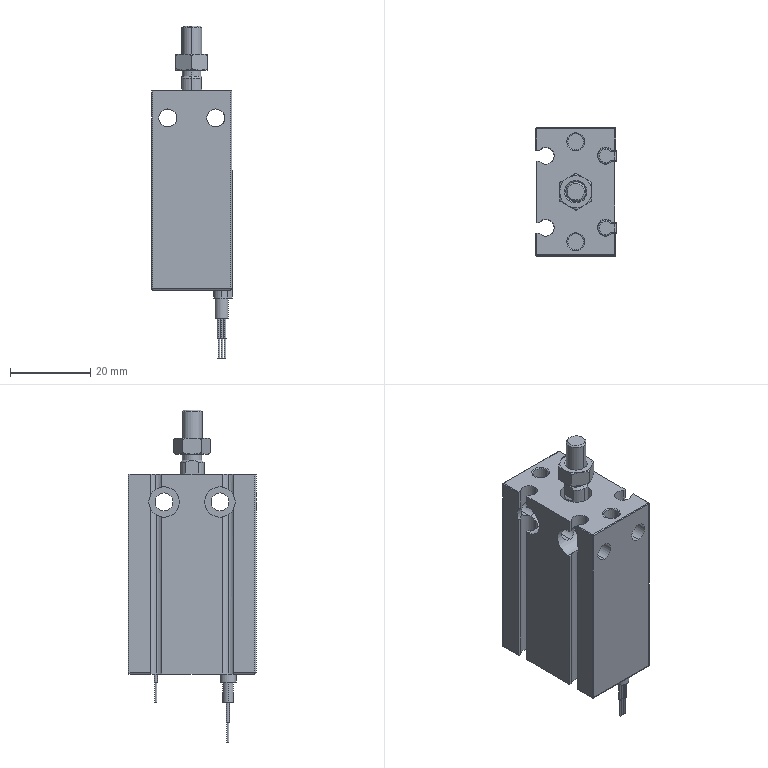Part | NX | features BREP 4 | 5 solids | 293 faces | box 20.11 x 32 x 83 mm | volume 25033 mm3 | cylinder 138 | plane 101 | torus 26 | cone 16 | sphere 8 | spline 4 | commonest cylinder face diameters 0.5 x28 7.6 x20 4.5 x16 4 x14 0.75 x12 2.05 x8